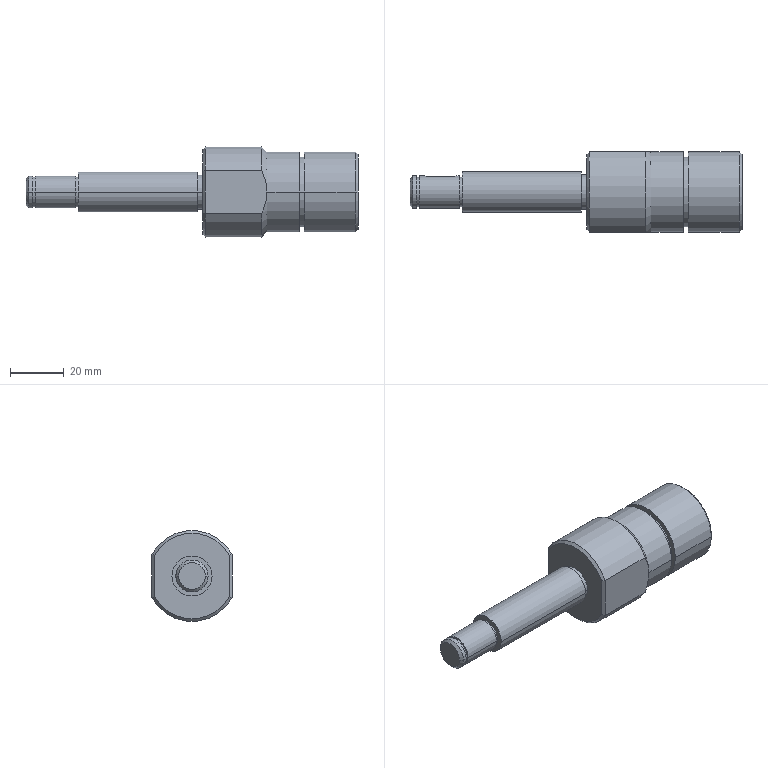Part | SolidWorks | features Chamfer 2, ICE 2, RevCut 1, Revolution 1 | 1 solid | 65 faces | box 124 x 30 x 34 mm | volume 43283 mm3 | cylinder 30 | plane 21 | cone 14 | commonest cylinder face diameters 11 x4 12 x4 19 x4 30 x4 4 x2 13 x2